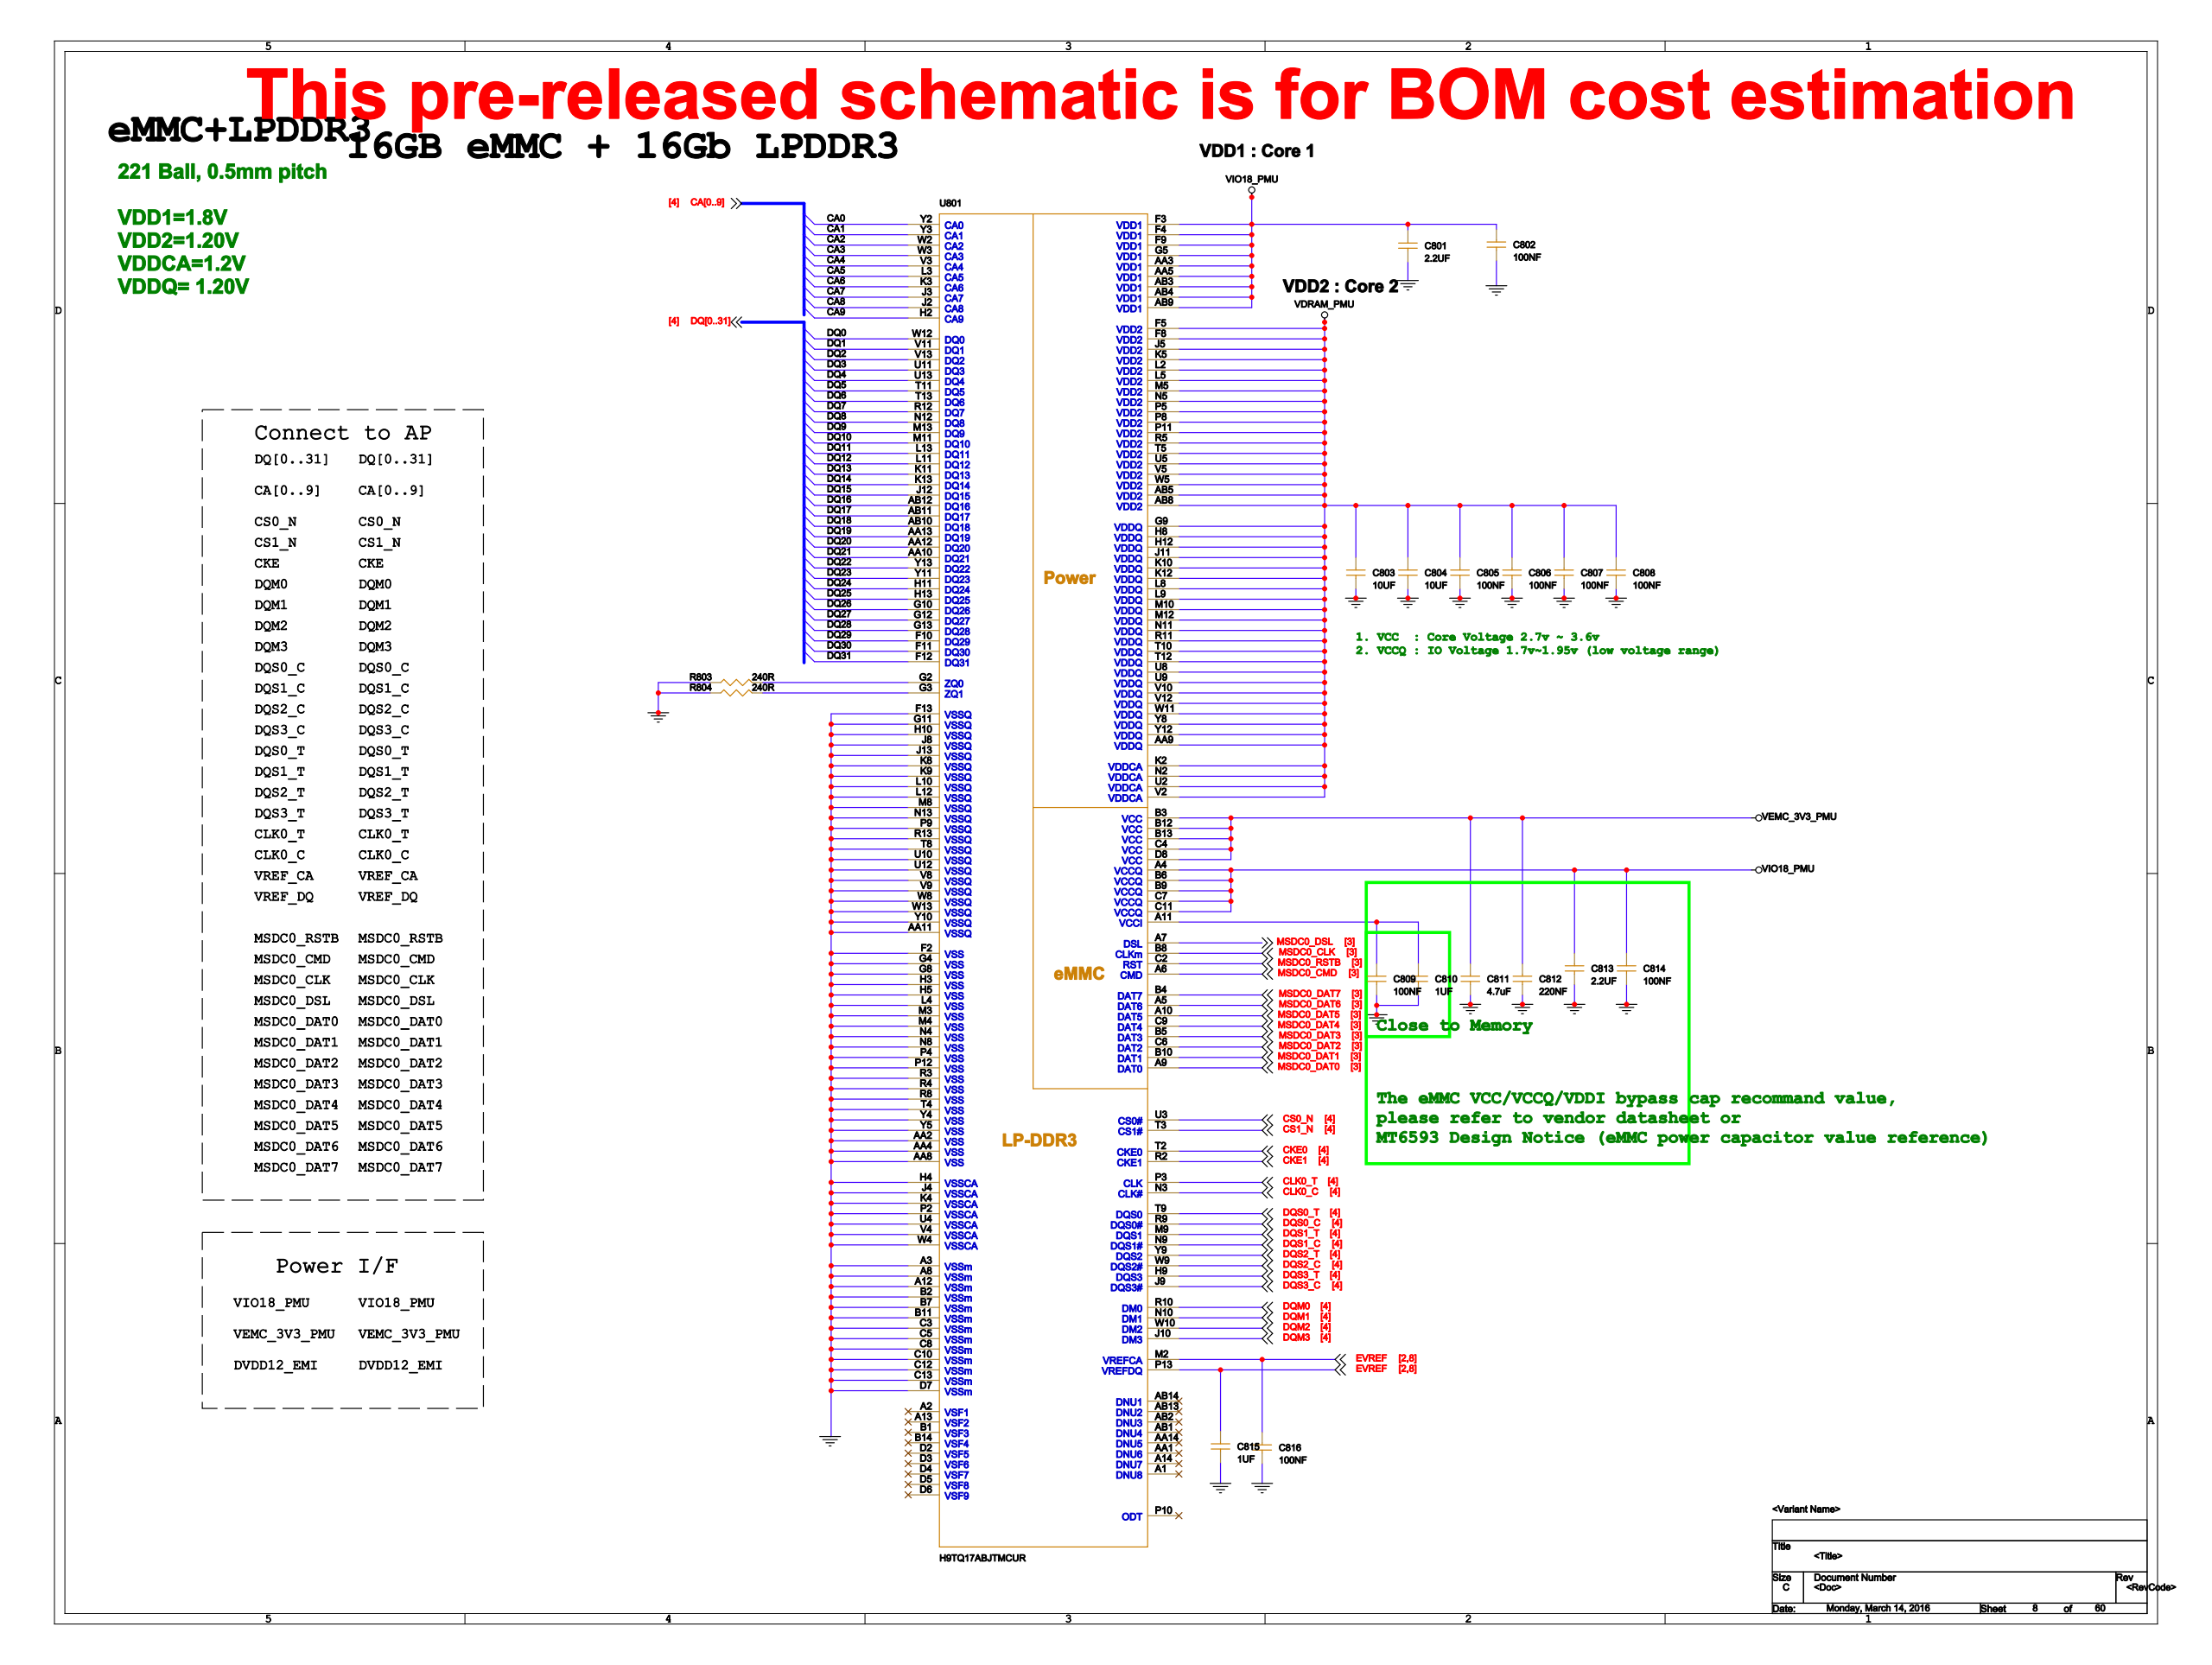Circuit board | Cadence Allegro | 1088 parts | 793 nets | one sheet of the schematic
Parts on this sheet (reference | value | footprint):
C801 | 2.2UF | 0402-BIG
C802 | 100NF | C0201
C803 | 10UF | 0402-BIG
C804 | 10UF | 0402-BIG
C805 | 100NF | C0201
C806 | 100NF | C0201
C807 | 100NF | C0201
C808 | 100NF | C0201
C809 | 100NF | C0201
C810 | 1UF | C0201
C811 | 4.7uF | 0402-BIG
C812 | 220NF | C0201
C813 | 2.2UF | 0402-BIG
C814 | 100NF | C0201
C815 | 1UF | C0201
C816 | 100NF | C0201
R803 | 240R | R0201
R804 | 240R | R0201
U801 | H9TQ17ABJTMCUR | BGA221_11P5X13X1P1_0P5
Nets of these parts (net: part-pin ...):
GND: C801-2 C802-2 C803-2 C804-2 C805-2 C806-2 C807-2 C808-2 C809-2 C810-2 C811-2 C812-2 C813-2 C814-2 C815-2 C816-2 R803-1 R804-1 U801-A3 U801-A8 U801-A12 U801-AA2 U801-AA4 U801-AA8 U801-AA11 U801-B2 U801-B7 U801-B11 U801-C3 U801-C5 U801-C8 U801-C10 U801-C12 U801-C13 U801-D7 U801-F2 U801-F13 U801-G4 U801-G8 U801-G11 U801-H3 U801-H4 U801-H5 U801-H10 U801-J4 U801-J8 U801-J13 U801-K4 U801-K8 U801-K9 U801-L4 U801-L10 U801-L12 U801-M3 U801-M4 U801-M8 U801-N4 U801-N8 U801-N13 U801-P2 U801-P4 U801-P9 U801-P12 U801-R3 U801-R4 U801-R8 U801-R13 U801-T4 U801-T8 U801-U4 U801-U10 U801-U12 U801-V4 U801-V8 U801-V9 U801-W4 U801-W8 U801-W13 U801-Y4 U801-Y5 U801-Y10
VDRAM_PMU: C803-1 C804-1 C805-1 C806-1 C807-1 C808-1 U801-AA9 U801-AB5 U801-AB8 U801-F5 U801-F8 U801-G9 U801-H8 U801-H12 U801-J5 U801-J11 U801-K2 U801-K5 U801-K10 U801-K12 U801-L2 U801-L5 U801-L8 U801-L9 U801-M5 U801-M10 U801-M12 U801-N2 U801-N5 U801-N11 U801-P5 U801-P8 U801-P11 U801-R5 U801-R11 U801-T5 U801-T10 U801-T12 U801-U2 U801-U5 U801-U8 U801-U9 U801-V2 U801-V5 U801-V10 U801-V12 U801-W5 U801-W11 U801-Y8 U801-Y12
EVREF: C815-1 C816-1 U801-M2 U801-P13
MSDC0_CLK: U801-B8
MSDC0_CMD: U801-A6
MSDC0_DAT0: U801-A9
MSDC0_DAT1: U801-B10
MSDC0_DAT2: U801-C6
MSDC0_DAT3: U801-B5
MSDC0_DAT4: U801-C9
MSDC0_DAT5: U801-A10
MSDC0_DAT6: U801-A5
MSDC0_DAT7: U801-B4
MSDC0_DSL: U801-A7
MSDC0_RSTB: U801-C2
VIO18_PMU: C801-1 C802-1 C813-1 C814-1 U801-A4 U801-AA3 U801-AA5 U801-AB3 U801-AB4 U801-AB9 U801-B6 U801-B9 U801-C7 U801-C11 U801-F3 U801-F4 U801-F9 U801-G5
CA0: U801-Y2
CA1: U801-Y3
CA2: U801-W2
CA3: U801-W3
CA4: U801-V3
CA5: U801-L3
CA6: U801-K3
CA7: U801-J3
CA8: U801-J2
CA9: U801-H2
CKE0: U801-T2
CKE1: U801-R2
CLK0_C: U801-N3
CLK0_T: U801-P3
CS0_N: U801-U3
CS1_N: U801-T3
DQ0: U801-W12
DQ1: U801-V11
DQ10: U801-M11
DQ11: U801-L13
DQ12: U801-L11
DQ13: U801-K11
DQ14: U801-K13
DQ15: U801-J12
DQ16: U801-AB12
DQ17: U801-AB11
DQ18: U801-AB10
DQ19: U801-AA13
DQ2: U801-V13
DQ20: U801-AA12
DQ21: U801-AA10
DQ22: U801-Y13
DQ23: U801-Y11
DQ24: U801-H11
DQ25: U801-H13
DQ26: U801-G10
DQ27: U801-G12
DQ28: U801-G13
DQ29: U801-F10
DQ3: U801-U11
DQ30: U801-F11
DQ31: U801-F12
DQ4: U801-U13
DQ5: U801-T11
DQ6: U801-T13
DQ7: U801-R12
DQ8: U801-N12
DQ9: U801-M13
DQM0: U801-R10
DQM1: U801-N10
DQM2: U801-W10
DQM3: U801-J10
DQS0_C: U801-R9
DQS0_T: U801-T9
DQS1_C: U801-N9
DQS1_T: U801-M9
DQS2_C: U801-W9
DQS2_T: U801-Y9
DQS3_C: U801-J9
DQS3_T: U801-H9
VEMC_3V3_PMU: C811-1 C812-1 U801-B3 U801-B12 U801-B13 U801-C4 U801-D8
N33635681: C809-1 C810-1 U801-A11
N33635770: R803-2 U801-G2
N33635772: R804-2 U801-G3